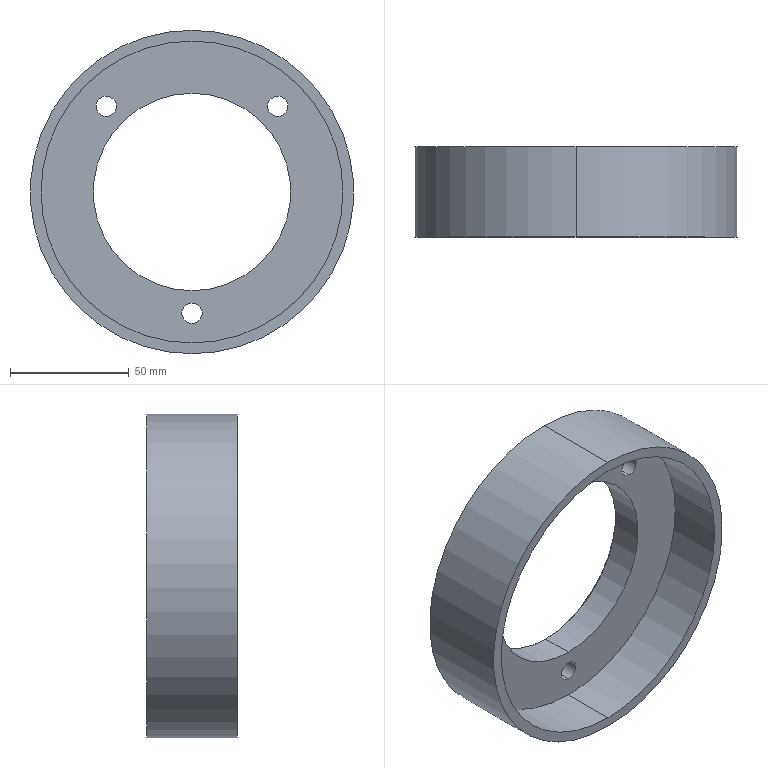Part | SolidWorks | features Chamfer 1, FlatPattern 1, HoleWzd 1, ICE 1, SMBaseFlange 1, SheetMetal 1 | 1 solid | 17 faces | box 136 x 38 x 136 mm | volume 173271 mm3 | cylinder 12 | plane 3 | cone 2 | commonest cylinder face diameters 8.5 x6 83 x2 127 x2 136 x2
STEP:
#1=CARTESIAN_POINT('',(0.,-1.,-41.5));
#2=VERTEX_POINT('',#1);
#3=CARTESIAN_POINT('',(0.,-1.,41.5));
#4=VERTEX_POINT('',#3);
#5=CARTESIAN_POINT('',(0.,-1.,0.));
#6=DIRECTION('',(0.,1.,0.));
#7=DIRECTION('',(0.,0.,1.));
#8=AXIS2_PLACEMENT_3D('',#5,#6,#7);
#9=CIRCLE('',#8,41.5);
#10=EDGE_CURVE('',#2,#4,#9,.T.);
#11=ORIENTED_EDGE('',*,*,#10,.F.);
#12=CARTESIAN_POINT('',(0.,0.,-42.5));
#13=VERTEX_POINT('',#12);
#14=CARTESIAN_POINT('',(0.,-1.,-41.5));
#15=DIRECTION('',(0.,0.7071,-0.7071));
#16=VECTOR('',#15,1000.);
#17=LINE('',#14,#16);
#18=EDGE_CURVE('',#2,#13,#17,.T.);
#19=ORIENTED_EDGE('',*,*,#18,.T.);
#20=CARTESIAN_POINT('',(0.,0.,42.5));
#21=VERTEX_POINT('',#20);
#22=CARTESIAN_POINT('',(0.,0.,0.));
#23=DIRECTION('',(0.,-1.,0.));
#24=DIRECTION('',(0.,0.,1.));
#25=AXIS2_PLACEMENT_3D('',#22,#23,#24);
#26=CIRCLE('',#25,42.5);
#27=EDGE_CURVE('',#21,#13,#26,.T.);
#28=ORIENTED_EDGE('',*,*,#27,.F.);
#29=CARTESIAN_POINT('',(0.,-1.,41.5));
#30=DIRECTION('',(0.,0.7071,0.7071));
#31=VECTOR('',#30,1000.);
#32=LINE('',#29,#31);
#33=EDGE_CURVE('',#4,#21,#32,.T.);
#34=ORIENTED_EDGE('',*,*,#33,.F.);
#35=EDGE_LOOP('',(#11,#19,#28,#34));
#36=FACE_OUTER_BOUND('',#35,.T.);
#37=CARTESIAN_POINT('',(0.,-1.,0.));
#38=DIRECTION('',(0.,1.,0.));
#39=DIRECTION('',(0.,0.,1.));
#40=AXIS2_PLACEMENT_3D('',#37,#38,#39);
#41=CONICAL_SURFACE('',#40,41.5,0.7854);
#42=ADVANCED_FACE('',(#36),#41,.F.);
#43=CARTESIAN_POINT('',(0.,-14.5,-46.75));
#44=VERTEX_POINT('',#43);
#45=CARTESIAN_POINT('',(0.,-14.5,-55.25));
#46=VERTEX_POINT('',#45);
#47=CARTESIAN_POINT('',(0.,-14.5,-51.));
#48=DIRECTION('',(0.,-1.,0.));
#49=DIRECTION('',(0.,0.,-1.));
#50=AXIS2_PLACEMENT_3D('',#47,#48,#49);
#51=CIRCLE('',#50,4.25);
#52=EDGE_CURVE('',#44,#46,#51,.T.);
#53=ORIENTED_EDGE('',*,*,#52,.T.);
#54=CARTESIAN_POINT('',(0.,0.,-55.25));
#55=VERTEX_POINT('',#54);
#56=CARTESIAN_POINT('',(0.,0.,-55.25));
#57=DIRECTION('',(0.,1.,0.));
#58=VECTOR('',#57,1000.);
#59=LINE('',#56,#58);
#60=EDGE_CURVE('',#46,#55,#59,.T.);
#61=ORIENTED_EDGE('',*,*,#60,.T.);
#62=CARTESIAN_POINT('',(0.,0.,-46.75));
#63=VERTEX_POINT('',#62);
#64=CARTESIAN_POINT('',(0.,0.,-51.));
#65=DIRECTION('',(0.,1.,0.));
#66=DIRECTION('',(0.,0.,1.));
#67=AXIS2_PLACEMENT_3D('',#64,#65,#66);
#68=CIRCLE('',#67,4.25);
#69=EDGE_CURVE('',#55,#63,#68,.T.);
#70=ORIENTED_EDGE('',*,*,#69,.T.);
#71=CARTESIAN_POINT('',(0.,0.,-46.75));
#72=DIRECTION('',(0.,1.,0.));
#73=VECTOR('',#72,1000.);
#74=LINE('',#71,#73);
#75=EDGE_CURVE('',#44,#63,#74,.T.);
#76=ORIENTED_EDGE('',*,*,#75,.F.);
#77=EDGE_LOOP('',(#53,#61,#70,#76));
#78=FACE_OUTER_BOUND('',#77,.T.);
#79=CARTESIAN_POINT('',(0.,0.,-51.));
#80=DIRECTION('',(0.,1.,0.));
#81=DIRECTION('',(0.,0.,1.));
#82=AXIS2_PLACEMENT_3D('',#79,#80,#81);
#83=CYLINDRICAL_SURFACE('',#82,4.25);
#84=ADVANCED_FACE('',(#78),#83,.F.);
#85=CARTESIAN_POINT('',(-36.062,-14.5,40.312));
#86=VERTEX_POINT('',#85);
#87=CARTESIAN_POINT('',(-36.062,-14.5,31.812));
#88=VERTEX_POINT('',#87);
#89=CARTESIAN_POINT('',(-36.062,-14.5,36.062));
#90=DIRECTION('',(0.,-1.,0.));
#91=DIRECTION('',(0.,0.,-1.));
#92=AXIS2_PLACEMENT_3D('',#89,#90,#91);
#93=CIRCLE('',#92,4.25);
#94=EDGE_CURVE('',#86,#88,#93,.T.);
#95=ORIENTED_EDGE('',*,*,#94,.T.);
#96=CARTESIAN_POINT('',(-36.062,0.,31.812));
#97=VERTEX_POINT('',#96);
#98=CARTESIAN_POINT('',(-36.062,0.,31.812));
#99=DIRECTION('',(0.,1.,0.));
#100=VECTOR('',#99,1000.);
#101=LINE('',#98,#100);
#102=EDGE_CURVE('',#88,#97,#101,.T.);
#103=ORIENTED_EDGE('',*,*,#102,.T.);
#104=CARTESIAN_POINT('',(-36.062,0.,40.312));
#105=VERTEX_POINT('',#104);
#106=CARTESIAN_POINT('',(-36.062,0.,36.062));
#107=DIRECTION('',(0.,1.,0.));
#108=DIRECTION('',(0.,0.,1.));
#109=AXIS2_PLACEMENT_3D('',#106,#107,#108);
#110=CIRCLE('',#109,4.25);
#111=EDGE_CURVE('',#97,#105,#110,.T.);
#112=ORIENTED_EDGE('',*,*,#111,.T.);
#113=CARTESIAN_POINT('',(-36.062,0.,40.312));
#114=DIRECTION('',(0.,1.,0.));
#115=VECTOR('',#114,1000.);
#116=LINE('',#113,#115);
#117=EDGE_CURVE('',#86,#105,#116,.T.);
#118=ORIENTED_EDGE('',*,*,#117,.F.);
#119=EDGE_LOOP('',(#95,#103,#112,#118));
#120=FACE_OUTER_BOUND('',#119,.T.);
#121=CARTESIAN_POINT('',(-36.062,0.,36.062));
#122=DIRECTION('',(0.,1.,0.));
#123=DIRECTION('',(0.,0.,1.));
#124=AXIS2_PLACEMENT_3D('',#121,#122,#123);
#125=CYLINDRICAL_SURFACE('',#124,4.25);
#126=ADVANCED_FACE('',(#120),#125,.F.);
#127=CARTESIAN_POINT('',(36.062,-14.5,40.312));
#128=VERTEX_POINT('',#127);
#129=CARTESIAN_POINT('',(36.062,-14.5,31.812));
#130=VERTEX_POINT('',#129);
#131=CARTESIAN_POINT('',(36.062,-14.5,36.062));
#132=DIRECTION('',(0.,-1.,0.));
#133=DIRECTION('',(0.,0.,-1.));
#134=AXIS2_PLACEMENT_3D('',#131,#132,#133);
#135=CIRCLE('',#134,4.25);
#136=EDGE_CURVE('',#128,#130,#135,.T.);
#137=ORIENTED_EDGE('',*,*,#136,.T.);
#138=CARTESIAN_POINT('',(36.062,0.,31.812));
#139=VERTEX_POINT('',#138);
#140=CARTESIAN_POINT('',(36.062,0.,31.812));
#141=DIRECTION('',(0.,1.,0.));
#142=VECTOR('',#141,1000.);
#143=LINE('',#140,#142);
#144=EDGE_CURVE('',#130,#139,#143,.T.);
#145=ORIENTED_EDGE('',*,*,#144,.T.);
#146=CARTESIAN_POINT('',(36.062,0.,40.312));
#147=VERTEX_POINT('',#146);
#148=CARTESIAN_POINT('',(36.062,0.,36.062));
#149=DIRECTION('',(0.,1.,0.));
#150=DIRECTION('',(0.,0.,1.));
#151=AXIS2_PLACEMENT_3D('',#148,#149,#150);
#152=CIRCLE('',#151,4.25);
#153=EDGE_CURVE('',#139,#147,#152,.T.);
#154=ORIENTED_EDGE('',*,*,#153,.T.);
#155=CARTESIAN_POINT('',(36.062,0.,40.312));
#156=DIRECTION('',(0.,1.,0.));
#157=VECTOR('',#156,1000.);
#158=LINE('',#155,#157);
#159=EDGE_CURVE('',#128,#147,#158,.T.);
#160=ORIENTED_EDGE('',*,*,#159,.F.);
#161=EDGE_LOOP('',(#137,#145,#154,#160));
#162=FACE_OUTER_BOUND('',#161,.T.);
#163=CARTESIAN_POINT('',(36.062,0.,36.062));
#164=DIRECTION('',(0.,1.,0.));
#165=DIRECTION('',(0.,0.,1.));
#166=AXIS2_PLACEMENT_3D('',#163,#164,#165);
#167=CYLINDRICAL_SURFACE('',#166,4.25);
#168=ADVANCED_FACE('',(#162),#167,.F.);
#169=CARTESIAN_POINT('',(0.,-14.5,63.5));
#170=VERTEX_POINT('',#169);
#171=CARTESIAN_POINT('',(0.,-14.5,-63.5));
#172=VERTEX_POINT('',#171);
#173=CARTESIAN_POINT('',(0.,-14.5,0.));
#174=DIRECTION('',(0.,-1.,0.));
#175=DIRECTION('',(0.,0.,-1.));
#176=AXIS2_PLACEMENT_3D('',#173,#174,#175);
#177=CIRCLE('',#176,63.5);
#178=EDGE_CURVE('',#170,#172,#177,.T.);
#179=ORIENTED_EDGE('',*,*,#178,.F.);
#180=CARTESIAN_POINT('',(0.,-38.,63.5));
#181=VERTEX_POINT('',#180);
#182=CARTESIAN_POINT('',(0.,-14.5,63.5));
#183=DIRECTION('',(0.,-1.,0.));
#184=VECTOR('',#183,1000.);
#185=LINE('',#182,#184);
#186=EDGE_CURVE('',#170,#181,#185,.T.);
#187=ORIENTED_EDGE('',*,*,#186,.T.);
#188=CARTESIAN_POINT('',(0.,-38.,-63.5));
#189=VERTEX_POINT('',#188);
#190=CARTESIAN_POINT('',(0.,-38.,0.));
#191=DIRECTION('',(0.,-1.,0.));
#192=DIRECTION('',(0.,0.,-1.));
#193=AXIS2_PLACEMENT_3D('',#190,#191,#192);
#194=CIRCLE('',#193,63.5);
#195=EDGE_CURVE('',#181,#189,#194,.T.);
#196=ORIENTED_EDGE('',*,*,#195,.T.);
#197=CARTESIAN_POINT('',(0.,-14.5,-63.5));
#198=DIRECTION('',(0.,-1.,0.));
#199=VECTOR('',#198,1000.);
#200=LINE('',#197,#199);
#201=EDGE_CURVE('',#172,#189,#200,.T.);
#202=ORIENTED_EDGE('',*,*,#201,.F.);
#203=EDGE_LOOP('',(#179,#187,#196,#202));
#204=FACE_OUTER_BOUND('',#203,.T.);
#205=CARTESIAN_POINT('',(0.,-14.5,0.));
#206=DIRECTION('',(0.,-1.,0.));
#207=DIRECTION('',(0.,0.,-1.));
#208=AXIS2_PLACEMENT_3D('',#205,#206,#207);
#209=CYLINDRICAL_SURFACE('',#208,63.5);
#210=ADVANCED_FACE('',(#204),#209,.F.);
#211=CARTESIAN_POINT('',(0.,-38.,68.));
#212=VERTEX_POINT('',#211);
#213=CARTESIAN_POINT('',(0.,-38.,-68.));
#214=VERTEX_POINT('',#213);
#215=CARTESIAN_POINT('',(0.,-38.,0.));
#216=DIRECTION('',(0.,1.,0.));
#217=DIRECTION('',(0.,0.,1.));
#218=AXIS2_PLACEMENT_3D('',#215,#216,#217);
#219=CIRCLE('',#218,68.);
#220=EDGE_CURVE('',#212,#214,#219,.T.);
#221=ORIENTED_EDGE('',*,*,#220,.T.);
#222=CARTESIAN_POINT('',(0.,0.,-68.));
#223=VERTEX_POINT('',#222);
#224=CARTESIAN_POINT('',(0.,-38.,-68.));
#225=DIRECTION('',(0.,1.,0.));
#226=VECTOR('',#225,1000.);
#227=LINE('',#224,#226);
#228=EDGE_CURVE('',#214,#223,#227,.T.);
#229=ORIENTED_EDGE('',*,*,#228,.T.);
#230=CARTESIAN_POINT('',(0.,0.,68.));
#231=VERTEX_POINT('',#230);
#232=CARTESIAN_POINT('',(0.,0.,0.));
#233=DIRECTION('',(0.,1.,0.));
#234=DIRECTION('',(0.,0.,1.));
#235=AXIS2_PLACEMENT_3D('',#232,#233,#234);
#236=CIRCLE('',#235,68.);
#237=EDGE_CURVE('',#231,#223,#236,.T.);
#238=ORIENTED_EDGE('',*,*,#237,.F.);
#239=CARTESIAN_POINT('',(0.,-38.,68.));
#240=DIRECTION('',(0.,1.,0.));
#241=VECTOR('',#240,1000.);
#242=LINE('',#239,#241);
#243=EDGE_CURVE('',#212,#231,#242,.T.);
#244=ORIENTED_EDGE('',*,*,#243,.F.);
#245=EDGE_LOOP('',(#221,#229,#238,#244));
#246=FACE_OUTER_BOUND('',#245,.T.);
#247=CARTESIAN_POINT('',(0.,-38.,0.));
#248=DIRECTION('',(0.,1.,0.));
#249=DIRECTION('',(0.,0.,1.));
#250=AXIS2_PLACEMENT_3D('',#247,#248,#249);
#251=CYLINDRICAL_SURFACE('',#250,68.);
#252=ADVANCED_FACE('',(#246),#251,.T.);
#253=CARTESIAN_POINT('',(0.,-14.5,-41.5));
#254=VERTEX_POINT('',#253);
#255=CARTESIAN_POINT('',(0.,-14.5,41.5));
#256=VERTEX_POINT('',#255);
#257=CARTESIAN_POINT('',(0.,-14.5,0.));
#258=DIRECTION('',(0.,1.,0.));
#259=DIRECTION('',(0.,0.,-1.));
#260=AXIS2_PLACEMENT_3D('',#257,#258,#259);
#261=CIRCLE('',#260,41.5);
#262=EDGE_CURVE('',#254,#256,#261,.T.);
#263=ORIENTED_EDGE('',*,*,#262,.F.);
#264=CARTESIAN_POINT('',(0.,-38.,-41.5));
#265=DIRECTION('',(0.,1.,0.));
#266=VECTOR('',#265,1000.);
#267=LINE('',#264,#266);
#268=EDGE_CURVE('',#254,#2,#267,.T.);
#269=ORIENTED_EDGE('',*,*,#268,.T.);
#270=ORIENTED_EDGE('',*,*,#10,.T.);
#271=CARTESIAN_POINT('',(0.,-38.,41.5));
#272=DIRECTION('',(0.,1.,0.));
#273=VECTOR('',#272,1000.);
#274=LINE('',#271,#273);
#275=EDGE_CURVE('',#256,#4,#274,.T.);
#276=ORIENTED_EDGE('',*,*,#275,.F.);
#277=EDGE_LOOP('',(#263,#269,#270,#276));
#278=FACE_OUTER_BOUND('',#277,.T.);
#279=CARTESIAN_POINT('',(0.,-38.,0.));
#280=DIRECTION('',(0.,1.,0.));
#281=DIRECTION('',(0.,0.,1.));
#282=AXIS2_PLACEMENT_3D('',#279,#280,#281);
#283=CYLINDRICAL_SURFACE('',#282,41.5);
#284=ADVANCED_FACE('',(#278),#283,.F.);
#285=ORIENTED_EDGE('',*,*,#268,.F.);
#286=CARTESIAN_POINT('',(0.,-14.5,0.));
#287=DIRECTION('',(0.,1.,0.));
#288=DIRECTION('',(0.,0.,-1.));
#289=AXIS2_PLACEMENT_3D('',#286,#287,#288);
#290=CIRCLE('',#289,41.5);
#291=EDGE_CURVE('',#256,#254,#290,.T.);
#292=ORIENTED_EDGE('',*,*,#291,.F.);
#293=ORIENTED_EDGE('',*,*,#275,.T.);
#294=CARTESIAN_POINT('',(0.,-1.,0.));
#295=DIRECTION('',(0.,1.,0.));
#296=DIRECTION('',(0.,0.,1.));
#297=AXIS2_PLACEMENT_3D('',#294,#295,#296);
#298=CIRCLE('',#297,41.5);
#299=EDGE_CURVE('',#4,#2,#298,.T.);
#300=ORIENTED_EDGE('',*,*,#299,.T.);
#301=EDGE_LOOP('',(#285,#292,#293,#300));
#302=FACE_OUTER_BOUND('',#301,.T.);
#303=CARTESIAN_POINT('',(0.,-38.,0.));
#304=DIRECTION('',(0.,1.,0.));
#305=DIRECTION('',(0.,0.,1.));
#306=AXIS2_PLACEMENT_3D('',#303,#304,#305);
#307=CYLINDRICAL_SURFACE('',#306,41.5);
#308=ADVANCED_FACE('',(#302),#307,.F.);
#309=ORIENTED_EDGE('',*,*,#228,.F.);
#310=CARTESIAN_POINT('',(0.,-38.,0.));
#311=DIRECTION('',(0.,1.,0.));
#312=DIRECTION('',(0.,0.,1.));
#313=AXIS2_PLACEMENT_3D('',#310,#311,#312);
#314=CIRCLE('',#313,68.);
#315=EDGE_CURVE('',#214,#212,#314,.T.);
#316=ORIENTED_EDGE('',*,*,#315,.T.);
#317=ORIENTED_EDGE('',*,*,#243,.T.);
#318=CARTESIAN_POINT('',(0.,0.,0.));
#319=DIRECTION('',(0.,1.,0.));
#320=DIRECTION('',(0.,0.,1.));
#321=AXIS2_PLACEMENT_3D('',#318,#319,#320);
#322=CIRCLE('',#321,68.);
#323=EDGE_CURVE('',#223,#231,#322,.T.);
#324=ORIENTED_EDGE('',*,*,#323,.F.);
#325=EDGE_LOOP('',(#309,#316,#317,#324));
#326=FACE_OUTER_BOUND('',#325,.T.);
#327=CARTESIAN_POINT('',(0.,-38.,0.));
#328=DIRECTION('',(0.,1.,0.));
#329=DIRECTION('',(0.,0.,1.));
#330=AXIS2_PLACEMENT_3D('',#327,#328,#329);
#331=CYLINDRICAL_SURFACE('',#330,68.);
#332=ADVANCED_FACE('',(#326),#331,.T.);
#333=CARTESIAN_POINT('',(0.,-38.,0.));
#334=DIRECTION('',(0.,-1.,0.));
#335=DIRECTION('',(0.,0.,-1.));
#336=AXIS2_PLACEMENT_3D('',#333,#334,#335);
#337=CIRCLE('',#336,63.5);
#338=EDGE_CURVE('',#189,#181,#337,.T.);
#339=ORIENTED_EDGE('',*,*,#338,.F.);
#340=ORIENTED_EDGE('',*,*,#195,.F.);
#341=EDGE_LOOP('',(#339,#340));
#342=FACE_BOUND('',#341,.T.);
#343=ORIENTED_EDGE('',*,*,#220,.F.);
#344=ORIENTED_EDGE('',*,*,#315,.F.);
#345=EDGE_LOOP('',(#343,#344));
#346=FACE_OUTER_BOUND('',#345,.T.);
#347=CARTESIAN_POINT('',(0.,-38.,0.));
#348=DIRECTION('',(0.,1.,0.));
#349=DIRECTION('',(0.,0.,1.));
#350=AXIS2_PLACEMENT_3D('',#347,#348,#349);
#351=PLANE('',#350);
#352=ADVANCED_FACE('',(#342,#346),#351,.F.);
#353=ORIENTED_EDGE('',*,*,#27,.T.);
#354=CARTESIAN_POINT('',(0.,0.,0.));
#355=DIRECTION('',(0.,-1.,0.));
#356=DIRECTION('',(0.,0.,1.));
#357=AXIS2_PLACEMENT_3D('',#354,#355,#356);
#358=CIRCLE('',#357,42.5);
#359=EDGE_CURVE('',#13,#21,#358,.T.);
#360=ORIENTED_EDGE('',*,*,#359,.T.);
#361=EDGE_LOOP('',(#353,#360));
#362=FACE_BOUND('',#361,.T.);
#363=CARTESIAN_POINT('',(0.,0.,-51.));
#364=DIRECTION('',(0.,1.,0.));
#365=DIRECTION('',(0.,0.,1.));
#366=AXIS2_PLACEMENT_3D('',#363,#364,#365);
#367=CIRCLE('',#366,4.25);
#368=EDGE_CURVE('',#63,#55,#367,.T.);
#369=ORIENTED_EDGE('',*,*,#368,.F.);
#370=ORIENTED_EDGE('',*,*,#69,.F.);
#371=EDGE_LOOP('',(#369,#370));
#372=FACE_BOUND('',#371,.T.);
#373=CARTESIAN_POINT('',(-36.062,0.,36.062));
#374=DIRECTION('',(0.,1.,0.));
#375=DIRECTION('',(0.,0.,1.));
#376=AXIS2_PLACEMENT_3D('',#373,#374,#375);
#377=CIRCLE('',#376,4.25);
#378=EDGE_CURVE('',#105,#97,#377,.T.);
#379=ORIENTED_EDGE('',*,*,#378,.F.);
#380=ORIENTED_EDGE('',*,*,#111,.F.);
#381=EDGE_LOOP('',(#379,#380));
#382=FACE_BOUND('',#381,.T.);
#383=CARTESIAN_POINT('',(36.062,0.,36.062));
#384=DIRECTION('',(0.,1.,0.));
#385=DIRECTION('',(0.,0.,1.));
#386=AXIS2_PLACEMENT_3D('',#383,#384,#385);
#387=CIRCLE('',#386,4.25);
#388=EDGE_CURVE('',#147,#139,#387,.T.);
#389=ORIENTED_EDGE('',*,*,#388,.F.);
#390=ORIENTED_EDGE('',*,*,#153,.F.);
#391=EDGE_LOOP('',(#389,#390));
#392=FACE_BOUND('',#391,.T.);
#393=ORIENTED_EDGE('',*,*,#237,.T.);
#394=ORIENTED_EDGE('',*,*,#323,.T.);
#395=EDGE_LOOP('',(#393,#394));
#396=FACE_OUTER_BOUND('',#395,.T.);
#397=CARTESIAN_POINT('',(0.,0.,0.));
#398=DIRECTION('',(0.,1.,0.));
#399=DIRECTION('',(0.,0.,1.));
#400=AXIS2_PLACEMENT_3D('',#397,#398,#399);
#401=PLANE('',#400);
#402=ADVANCED_FACE('',(#362,#372,#382,#392,#396),#401,.T.);
#403=ORIENTED_EDGE('',*,*,#52,.F.);
#404=CARTESIAN_POINT('',(0.,-14.5,-51.));
#405=DIRECTION('',(0.,-1.,0.));
#406=DIRECTION('',(0.,0.,-1.));
#407=AXIS2_PLACEMENT_3D('',#404,#405,#406);
#408=CIRCLE('',#407,4.25);
#409=EDGE_CURVE('',#46,#44,#408,.T.);
#410=ORIENTED_EDGE('',*,*,#409,.F.);
#411=EDGE_LOOP('',(#403,#410));
#412=FACE_BOUND('',#411,.T.);
#413=ORIENTED_EDGE('',*,*,#94,.F.);
#414=CARTESIAN_POINT('',(-36.062,-14.5,36.062));
#415=DIRECTION('',(0.,-1.,0.));
#416=DIRECTION('',(0.,0.,-1.));
#417=AXIS2_PLACEMENT_3D('',#414,#415,#416);
#418=CIRCLE('',#417,4.25);
#419=EDGE_CURVE('',#88,#86,#418,.T.);
#420=ORIENTED_EDGE('',*,*,#419,.F.);
#421=EDGE_LOOP('',(#413,#420));
#422=FACE_BOUND('',#421,.T.);
#423=ORIENTED_EDGE('',*,*,#136,.F.);
#424=CARTESIAN_POINT('',(36.062,-14.5,36.062));
#425=DIRECTION('',(0.,-1.,0.));
#426=DIRECTION('',(0.,0.,-1.));
#427=AXIS2_PLACEMENT_3D('',#424,#425,#426);
#428=CIRCLE('',#427,4.25);
#429=EDGE_CURVE('',#130,#128,#428,.T.);
#430=ORIENTED_EDGE('',*,*,#429,.F.);
#431=EDGE_LOOP('',(#423,#430));
#432=FACE_BOUND('',#431,.T.);
#433=CARTESIAN_POINT('',(0.,-14.5,0.));
#434=DIRECTION('',(0.,-1.,0.));
#435=DIRECTION('',(0.,0.,-1.));
#436=AXIS2_PLACEMENT_3D('',#433,#434,#435);
#437=CIRCLE('',#436,63.5);
#438=EDGE_CURVE('',#172,#170,#437,.T.);
#439=ORIENTED_EDGE('',*,*,#438,.T.);
#440=ORIENTED_EDGE('',*,*,#178,.T.);
#441=EDGE_LOOP('',(#439,#440));
#442=FACE_OUTER_BOUND('',#441,.T.);
#443=ORIENTED_EDGE('',*,*,#291,.T.);
#444=ORIENTED_EDGE('',*,*,#262,.T.);
#445=EDGE_LOOP('',(#443,#444));
#446=FACE_BOUND('',#445,.T.);
#447=CARTESIAN_POINT('',(0.,-14.5,0.));
#448=DIRECTION('',(0.,-1.,0.));
#449=DIRECTION('',(0.,0.,-1.));
#450=AXIS2_PLACEMENT_3D('',#447,#448,#449);
#451=PLANE('',#450);
#452=ADVANCED_FACE('',(#412,#422,#432,#442,#446),#451,.T.);
#453=ORIENTED_EDGE('',*,*,#186,.F.);
#454=ORIENTED_EDGE('',*,*,#438,.F.);
#455=ORIENTED_EDGE('',*,*,#201,.T.);
#456=ORIENTED_EDGE('',*,*,#338,.T.);
#457=EDGE_LOOP('',(#453,#454,#455,#456));
#458=FACE_OUTER_BOUND('',#457,.T.);
#459=CARTESIAN_POINT('',(0.,-14.5,0.));
#460=DIRECTION('',(0.,-1.,0.));
#461=DIRECTION('',(0.,0.,-1.));
#462=AXIS2_PLACEMENT_3D('',#459,#460,#461);
#463=CYLINDRICAL_SURFACE('',#462,63.5);
#464=ADVANCED_FACE('',(#458),#463,.F.);
#465=ORIENTED_EDGE('',*,*,#144,.F.);
#466=ORIENTED_EDGE('',*,*,#429,.T.);
#467=ORIENTED_EDGE('',*,*,#159,.T.);
#468=ORIENTED_EDGE('',*,*,#388,.T.);
#469=EDGE_LOOP('',(#465,#466,#467,#468));
#470=FACE_OUTER_BOUND('',#469,.T.);
#471=CARTESIAN_POINT('',(36.062,0.,36.062));
#472=DIRECTION('',(0.,1.,0.));
#473=DIRECTION('',(0.,0.,1.));
#474=AXIS2_PLACEMENT_3D('',#471,#472,#473);
#475=CYLINDRICAL_SURFACE('',#474,4.25);
#476=ADVANCED_FACE('',(#470),#475,.F.);
#477=ORIENTED_EDGE('',*,*,#102,.F.);
#478=ORIENTED_EDGE('',*,*,#419,.T.);
#479=ORIENTED_EDGE('',*,*,#117,.T.);
#480=ORIENTED_EDGE('',*,*,#378,.T.);
#481=EDGE_LOOP('',(#477,#478,#479,#480));
#482=FACE_OUTER_BOUND('',#481,.T.);
#483=CARTESIAN_POINT('',(-36.062,0.,36.062));
#484=DIRECTION('',(0.,1.,0.));
#485=DIRECTION('',(0.,0.,1.));
#486=AXIS2_PLACEMENT_3D('',#483,#484,#485);
#487=CYLINDRICAL_SURFACE('',#486,4.25);
#488=ADVANCED_FACE('',(#482),#487,.F.);
#489=ORIENTED_EDGE('',*,*,#60,.F.);
#490=ORIENTED_EDGE('',*,*,#409,.T.);
#491=ORIENTED_EDGE('',*,*,#75,.T.);
#492=ORIENTED_EDGE('',*,*,#368,.T.);
#493=EDGE_LOOP('',(#489,#490,#491,#492));
#494=FACE_OUTER_BOUND('',#493,.T.);
#495=CARTESIAN_POINT('',(0.,0.,-51.));
#496=DIRECTION('',(0.,1.,0.));
#497=DIRECTION('',(0.,0.,1.));
#498=AXIS2_PLACEMENT_3D('',#495,#496,#497);
#499=CYLINDRICAL_SURFACE('',#498,4.25);
#500=ADVANCED_FACE('',(#494),#499,.F.);
#501=ORIENTED_EDGE('',*,*,#18,.F.);
#502=ORIENTED_EDGE('',*,*,#299,.F.);
#503=ORIENTED_EDGE('',*,*,#33,.T.);
#504=ORIENTED_EDGE('',*,*,#359,.F.);
#505=EDGE_LOOP('',(#501,#502,#503,#504));
#506=FACE_OUTER_BOUND('',#505,.T.);
#507=CARTESIAN_POINT('',(0.,-1.,0.));
#508=DIRECTION('',(0.,1.,0.));
#509=DIRECTION('',(0.,0.,1.));
#510=AXIS2_PLACEMENT_3D('',#507,#508,#509);
#511=CONICAL_SURFACE('',#510,41.5,0.7854);
#512=ADVANCED_FACE('',(#506),#511,.F.);
#513=CLOSED_SHELL('',(#42,#84,#126,#168,#210,#252,#284,#308,#332,#352,#402,#452,#464,#476,#488,#500,#512));
#514=MANIFOLD_SOLID_BREP('',#513);
#515=CARTESIAN_POINT('',(0.,0.,0.));
#516=DIRECTION('',(0.,0.,1.));
#517=DIRECTION('',(1.,0.,0.));
#518=AXIS2_PLACEMENT_3D('',#515,#516,#517);
#519=(LENGTH_UNIT()NAMED_UNIT(*)SI_UNIT(.MILLI.,.METRE.));
#520=UNCERTAINTY_MEASURE_WITH_UNIT(LENGTH_MEASURE(0.00001),#519,'','');
#521=(NAMED_UNIT(*)PLANE_ANGLE_UNIT()SI_UNIT($,.RADIAN.));
#522=(NAMED_UNIT(*)SI_UNIT($,.STERADIAN.)SOLID_ANGLE_UNIT());
#523=(GEOMETRIC_REPRESENTATION_CONTEXT(3)GLOBAL_UNCERTAINTY_ASSIGNED_CONTEXT((#520))GLOBAL_UNIT_ASSIGNED_CONTEXT((#519,#521,#522))REPRESENTATION_CONTEXT('',''));
#524=ADVANCED_BREP_SHAPE_REPRESENTATION('',(#514,#518),#523);